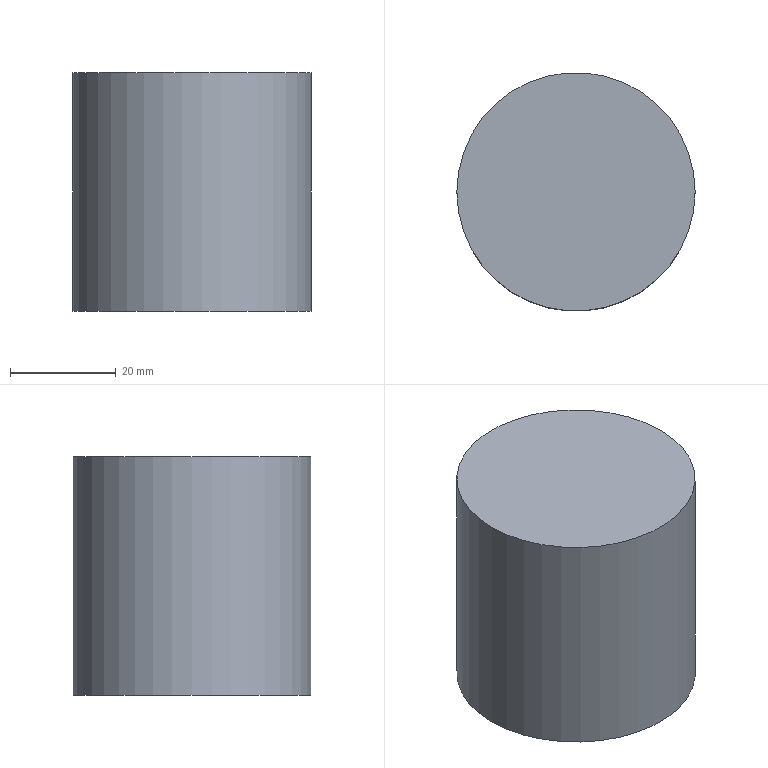Part | NX | features solid 2 | 1 solid | 3 faces | box 45 x 45 x 45 mm | volume 71569 mm3 | plane 2 | cylinder 1 | commonest cylinder face diameters 45 x1
STEP:
#1=CARTESIAN_POINT('',(-1207.5,660.,-65.));
#2=VERTEX_POINT('',#1);
#3=CARTESIAN_POINT('',(-1185.,660.,-65.));
#4=DIRECTION('',(0.,0.,1.));
#5=DIRECTION('',(-1.,0.,0.));
#6=AXIS2_PLACEMENT_3D('',#3,#4,#5);
#7=CIRCLE('',#6,22.5);
#8=EDGE_CURVE('',#2,#2,#7,.F.);
#9=ORIENTED_EDGE('',*,*,#8,.F.);
#10=EDGE_LOOP('',(#9));
#11=FACE_BOUND('',#10,.T.);
#12=CARTESIAN_POINT('',(-1207.5,660.,-20.));
#13=VERTEX_POINT('',#12);
#14=CARTESIAN_POINT('',(-1185.,660.,-20.));
#15=DIRECTION('',(0.,0.,1.));
#16=DIRECTION('',(-1.,0.,0.));
#17=AXIS2_PLACEMENT_3D('',#14,#15,#16);
#18=CIRCLE('',#17,22.5);
#19=EDGE_CURVE('',#13,#13,#18,.F.);
#20=ORIENTED_EDGE('',*,*,#19,.T.);
#21=EDGE_LOOP('',(#20));
#22=FACE_BOUND('',#21,.T.);
#23=CARTESIAN_POINT('',(-1185.,660.,-73.));
#24=DIRECTION('',(0.,0.,1.));
#25=DIRECTION('',(-1.,0.,0.));
#26=AXIS2_PLACEMENT_3D('',#23,#24,#25);
#27=CYLINDRICAL_SURFACE('',#26,22.5);
#28=ADVANCED_FACE('',(#11,#22),#27,.T.);
#29=ORIENTED_EDGE('',*,*,#8,.T.);
#30=EDGE_LOOP('',(#29));
#31=FACE_BOUND('',#30,.T.);
#32=CARTESIAN_POINT('',(-1185.,668.25,-65.));
#33=DIRECTION('',(0.,0.,1.));
#34=DIRECTION('',(1.,0.,0.));
#35=AXIS2_PLACEMENT_3D('',#32,#33,#34);
#36=PLANE('',#35);
#37=ADVANCED_FACE('',(#31),#36,.F.);
#38=ORIENTED_EDGE('',*,*,#19,.F.);
#39=EDGE_LOOP('',(#38));
#40=FACE_BOUND('',#39,.T.);
#41=CARTESIAN_POINT('',(-1185.,668.25,-20.));
#42=DIRECTION('',(0.,0.,1.));
#43=DIRECTION('',(1.,0.,0.));
#44=AXIS2_PLACEMENT_3D('',#41,#42,#43);
#45=PLANE('',#44);
#46=ADVANCED_FACE('',(#40),#45,.T.);
#47=CLOSED_SHELL('',(#28,#37,#46));
#48=MANIFOLD_SOLID_BREP('',#47);
#49=(LENGTH_UNIT()NAMED_UNIT(*)SI_UNIT(.MILLI.,.METRE.));
#50=UNCERTAINTY_MEASURE_WITH_UNIT(LENGTH_MEASURE(0.00001),#49,'','');
#51=(NAMED_UNIT(*)PLANE_ANGLE_UNIT()SI_UNIT($,.RADIAN.));
#52=(NAMED_UNIT(*)SI_UNIT($,.STERADIAN.)SOLID_ANGLE_UNIT());
#53=(GEOMETRIC_REPRESENTATION_CONTEXT(3)GLOBAL_UNCERTAINTY_ASSIGNED_CONTEXT((#50))GLOBAL_UNIT_ASSIGNED_CONTEXT((#49,#51,#52))REPRESENTATION_CONTEXT('',''));
#54=ADVANCED_BREP_SHAPE_REPRESENTATION('',(#48),#53);